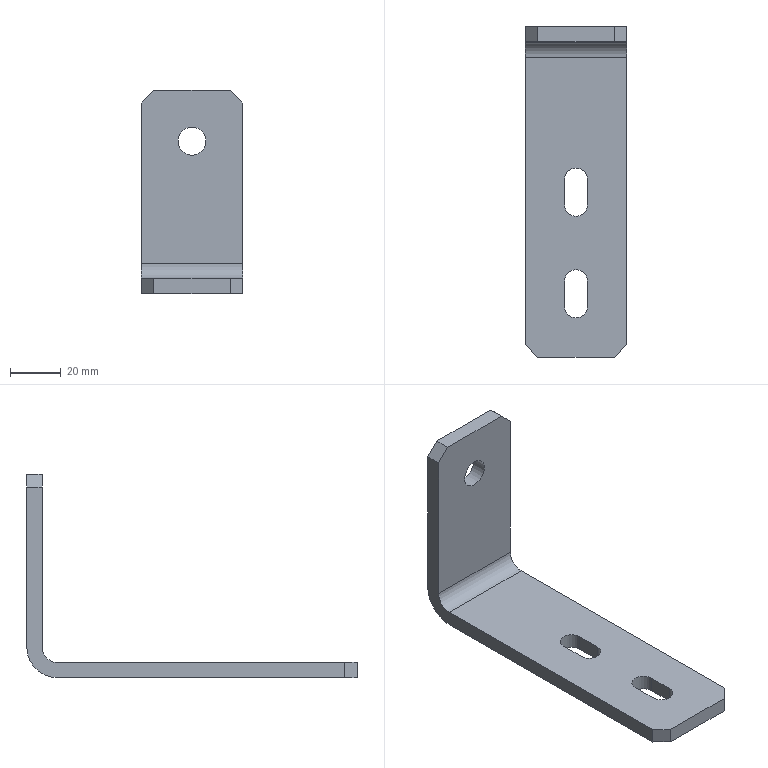Part | STEP file | support for guide1 | 1 solid | 23 faces | box 40 x 130 x 80 mm | volume 45319 mm3 | plane 16 | cylinder 6 | spline 1 | commonest cylinder face diameters 9 x4 12 x1 24 x1